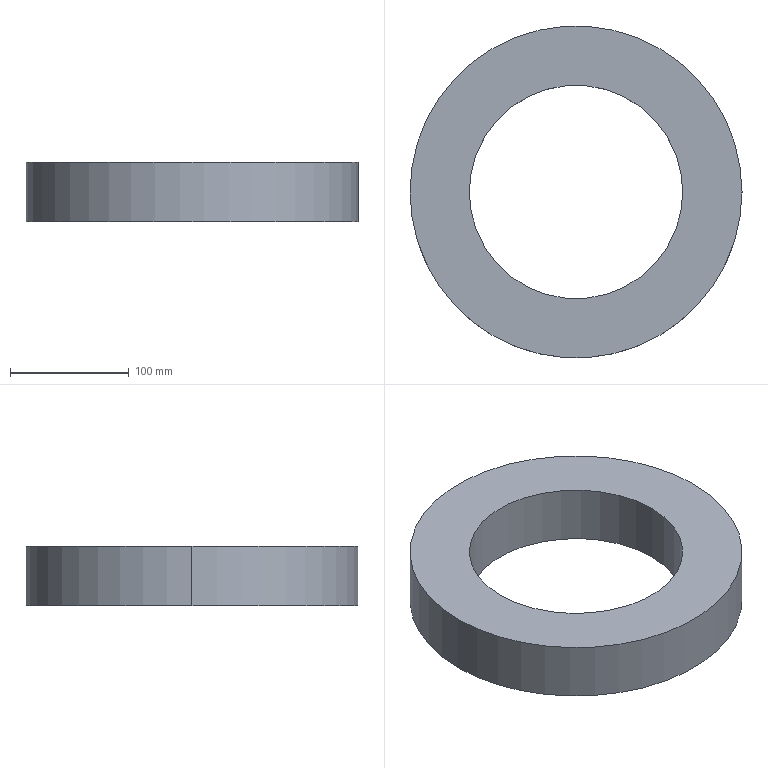Part | SolidWorks | features Extrusion 1 | 1 solid | 6 faces | box 280 x 280 x 50 mm | volume 1806416 mm3 | cylinder 4 | plane 2 | commonest cylinder face diameters 180 x2 280 x2
STEP:
#1=CARTESIAN_POINT('',(-90.,0.,-25.));
#2=VERTEX_POINT('',#1);
#3=CARTESIAN_POINT('',(90.,0.,-25.));
#4=VERTEX_POINT('',#3);
#5=CARTESIAN_POINT('',(0.,0.,-25.));
#6=DIRECTION('',(0.,0.,1.));
#7=DIRECTION('',(1.,0.,0.));
#8=AXIS2_PLACEMENT_3D('',#5,#6,#7);
#9=CIRCLE('',#8,90.);
#10=EDGE_CURVE('',#2,#4,#9,.T.);
#11=ORIENTED_EDGE('',*,*,#10,.F.);
#12=CARTESIAN_POINT('',(-90.,0.,25.));
#13=VERTEX_POINT('',#12);
#14=CARTESIAN_POINT('',(-90.,0.,-25.));
#15=DIRECTION('',(0.,0.,1.));
#16=VECTOR('',#15,1000.);
#17=LINE('',#14,#16);
#18=EDGE_CURVE('',#2,#13,#17,.T.);
#19=ORIENTED_EDGE('',*,*,#18,.T.);
#20=CARTESIAN_POINT('',(90.,0.,25.));
#21=VERTEX_POINT('',#20);
#22=CARTESIAN_POINT('',(0.,0.,25.));
#23=DIRECTION('',(0.,0.,1.));
#24=DIRECTION('',(1.,0.,0.));
#25=AXIS2_PLACEMENT_3D('',#22,#23,#24);
#26=CIRCLE('',#25,90.);
#27=EDGE_CURVE('',#13,#21,#26,.T.);
#28=ORIENTED_EDGE('',*,*,#27,.T.);
#29=CARTESIAN_POINT('',(90.,0.,-25.));
#30=DIRECTION('',(0.,0.,1.));
#31=VECTOR('',#30,1000.);
#32=LINE('',#29,#31);
#33=EDGE_CURVE('',#4,#21,#32,.T.);
#34=ORIENTED_EDGE('',*,*,#33,.F.);
#35=EDGE_LOOP('',(#11,#19,#28,#34));
#36=FACE_OUTER_BOUND('',#35,.T.);
#37=CARTESIAN_POINT('',(0.,0.,-25.));
#38=DIRECTION('',(0.,0.,1.));
#39=DIRECTION('',(1.,0.,0.));
#40=AXIS2_PLACEMENT_3D('',#37,#38,#39);
#41=CYLINDRICAL_SURFACE('',#40,90.);
#42=ADVANCED_FACE('',(#36),#41,.F.);
#43=CARTESIAN_POINT('',(140.,0.,-25.));
#44=VERTEX_POINT('',#43);
#45=CARTESIAN_POINT('',(-140.,0.,-25.));
#46=VERTEX_POINT('',#45);
#47=CARTESIAN_POINT('',(0.,0.,-25.));
#48=DIRECTION('',(0.,0.,1.));
#49=DIRECTION('',(1.,0.,0.));
#50=AXIS2_PLACEMENT_3D('',#47,#48,#49);
#51=CIRCLE('',#50,140.);
#52=EDGE_CURVE('',#44,#46,#51,.T.);
#53=ORIENTED_EDGE('',*,*,#52,.T.);
#54=CARTESIAN_POINT('',(-140.,0.,25.));
#55=VERTEX_POINT('',#54);
#56=CARTESIAN_POINT('',(-140.,0.,-25.));
#57=DIRECTION('',(0.,0.,1.));
#58=VECTOR('',#57,1000.);
#59=LINE('',#56,#58);
#60=EDGE_CURVE('',#46,#55,#59,.T.);
#61=ORIENTED_EDGE('',*,*,#60,.T.);
#62=CARTESIAN_POINT('',(140.,0.,25.));
#63=VERTEX_POINT('',#62);
#64=CARTESIAN_POINT('',(0.,0.,25.));
#65=DIRECTION('',(0.,0.,1.));
#66=DIRECTION('',(1.,0.,0.));
#67=AXIS2_PLACEMENT_3D('',#64,#65,#66);
#68=CIRCLE('',#67,140.);
#69=EDGE_CURVE('',#63,#55,#68,.T.);
#70=ORIENTED_EDGE('',*,*,#69,.F.);
#71=CARTESIAN_POINT('',(140.,0.,-25.));
#72=DIRECTION('',(0.,0.,1.));
#73=VECTOR('',#72,1000.);
#74=LINE('',#71,#73);
#75=EDGE_CURVE('',#44,#63,#74,.T.);
#76=ORIENTED_EDGE('',*,*,#75,.F.);
#77=EDGE_LOOP('',(#53,#61,#70,#76));
#78=FACE_OUTER_BOUND('',#77,.T.);
#79=CARTESIAN_POINT('',(0.,0.,-25.));
#80=DIRECTION('',(0.,0.,1.));
#81=DIRECTION('',(1.,0.,0.));
#82=AXIS2_PLACEMENT_3D('',#79,#80,#81);
#83=CYLINDRICAL_SURFACE('',#82,140.);
#84=ADVANCED_FACE('',(#78),#83,.T.);
#85=ORIENTED_EDGE('',*,*,#60,.F.);
#86=CARTESIAN_POINT('',(0.,0.,-25.));
#87=DIRECTION('',(0.,0.,1.));
#88=DIRECTION('',(1.,0.,0.));
#89=AXIS2_PLACEMENT_3D('',#86,#87,#88);
#90=CIRCLE('',#89,140.);
#91=EDGE_CURVE('',#46,#44,#90,.T.);
#92=ORIENTED_EDGE('',*,*,#91,.T.);
#93=ORIENTED_EDGE('',*,*,#75,.T.);
#94=CARTESIAN_POINT('',(0.,0.,25.));
#95=DIRECTION('',(0.,0.,1.));
#96=DIRECTION('',(1.,0.,0.));
#97=AXIS2_PLACEMENT_3D('',#94,#95,#96);
#98=CIRCLE('',#97,140.);
#99=EDGE_CURVE('',#55,#63,#98,.T.);
#100=ORIENTED_EDGE('',*,*,#99,.F.);
#101=EDGE_LOOP('',(#85,#92,#93,#100));
#102=FACE_OUTER_BOUND('',#101,.T.);
#103=CARTESIAN_POINT('',(0.,0.,-25.));
#104=DIRECTION('',(0.,0.,1.));
#105=DIRECTION('',(1.,0.,0.));
#106=AXIS2_PLACEMENT_3D('',#103,#104,#105);
#107=CYLINDRICAL_SURFACE('',#106,140.);
#108=ADVANCED_FACE('',(#102),#107,.T.);
#109=CARTESIAN_POINT('',(0.,0.,-25.));
#110=DIRECTION('',(0.,0.,1.));
#111=DIRECTION('',(1.,0.,0.));
#112=AXIS2_PLACEMENT_3D('',#109,#110,#111);
#113=CIRCLE('',#112,90.);
#114=EDGE_CURVE('',#4,#2,#113,.T.);
#115=ORIENTED_EDGE('',*,*,#114,.T.);
#116=ORIENTED_EDGE('',*,*,#10,.T.);
#117=EDGE_LOOP('',(#115,#116));
#118=FACE_BOUND('',#117,.T.);
#119=ORIENTED_EDGE('',*,*,#52,.F.);
#120=ORIENTED_EDGE('',*,*,#91,.F.);
#121=EDGE_LOOP('',(#119,#120));
#122=FACE_OUTER_BOUND('',#121,.T.);
#123=CARTESIAN_POINT('',(0.,0.,-25.));
#124=DIRECTION('',(0.,0.,1.));
#125=DIRECTION('',(1.,0.,0.));
#126=AXIS2_PLACEMENT_3D('',#123,#124,#125);
#127=PLANE('',#126);
#128=ADVANCED_FACE('',(#118,#122),#127,.F.);
#129=CARTESIAN_POINT('',(0.,0.,25.));
#130=DIRECTION('',(0.,0.,1.));
#131=DIRECTION('',(1.,0.,0.));
#132=AXIS2_PLACEMENT_3D('',#129,#130,#131);
#133=CIRCLE('',#132,90.);
#134=EDGE_CURVE('',#21,#13,#133,.T.);
#135=ORIENTED_EDGE('',*,*,#134,.F.);
#136=ORIENTED_EDGE('',*,*,#27,.F.);
#137=EDGE_LOOP('',(#135,#136));
#138=FACE_BOUND('',#137,.T.);
#139=ORIENTED_EDGE('',*,*,#69,.T.);
#140=ORIENTED_EDGE('',*,*,#99,.T.);
#141=EDGE_LOOP('',(#139,#140));
#142=FACE_OUTER_BOUND('',#141,.T.);
#143=CARTESIAN_POINT('',(0.,0.,25.));
#144=DIRECTION('',(0.,0.,1.));
#145=DIRECTION('',(1.,0.,0.));
#146=AXIS2_PLACEMENT_3D('',#143,#144,#145);
#147=PLANE('',#146);
#148=ADVANCED_FACE('',(#138,#142),#147,.T.);
#149=ORIENTED_EDGE('',*,*,#18,.F.);
#150=ORIENTED_EDGE('',*,*,#114,.F.);
#151=ORIENTED_EDGE('',*,*,#33,.T.);
#152=ORIENTED_EDGE('',*,*,#134,.T.);
#153=EDGE_LOOP('',(#149,#150,#151,#152));
#154=FACE_OUTER_BOUND('',#153,.T.);
#155=CARTESIAN_POINT('',(0.,0.,-25.));
#156=DIRECTION('',(0.,0.,1.));
#157=DIRECTION('',(1.,0.,0.));
#158=AXIS2_PLACEMENT_3D('',#155,#156,#157);
#159=CYLINDRICAL_SURFACE('',#158,90.);
#160=ADVANCED_FACE('',(#154),#159,.F.);
#161=CLOSED_SHELL('',(#42,#84,#108,#128,#148,#160));
#162=MANIFOLD_SOLID_BREP('',#161);
#163=CARTESIAN_POINT('',(0.,0.,0.));
#164=DIRECTION('',(0.,0.,1.));
#165=DIRECTION('',(1.,0.,0.));
#166=AXIS2_PLACEMENT_3D('',#163,#164,#165);
#167=(LENGTH_UNIT()NAMED_UNIT(*)SI_UNIT(.MILLI.,.METRE.));
#168=UNCERTAINTY_MEASURE_WITH_UNIT(LENGTH_MEASURE(0.00001),#167,'','');
#169=(NAMED_UNIT(*)PLANE_ANGLE_UNIT()SI_UNIT($,.RADIAN.));
#170=(NAMED_UNIT(*)SI_UNIT($,.STERADIAN.)SOLID_ANGLE_UNIT());
#171=(GEOMETRIC_REPRESENTATION_CONTEXT(3)GLOBAL_UNCERTAINTY_ASSIGNED_CONTEXT((#168))GLOBAL_UNIT_ASSIGNED_CONTEXT((#167,#169,#170))REPRESENTATION_CONTEXT('',''));
#172=ADVANCED_BREP_SHAPE_REPRESENTATION('',(#162,#166),#171);